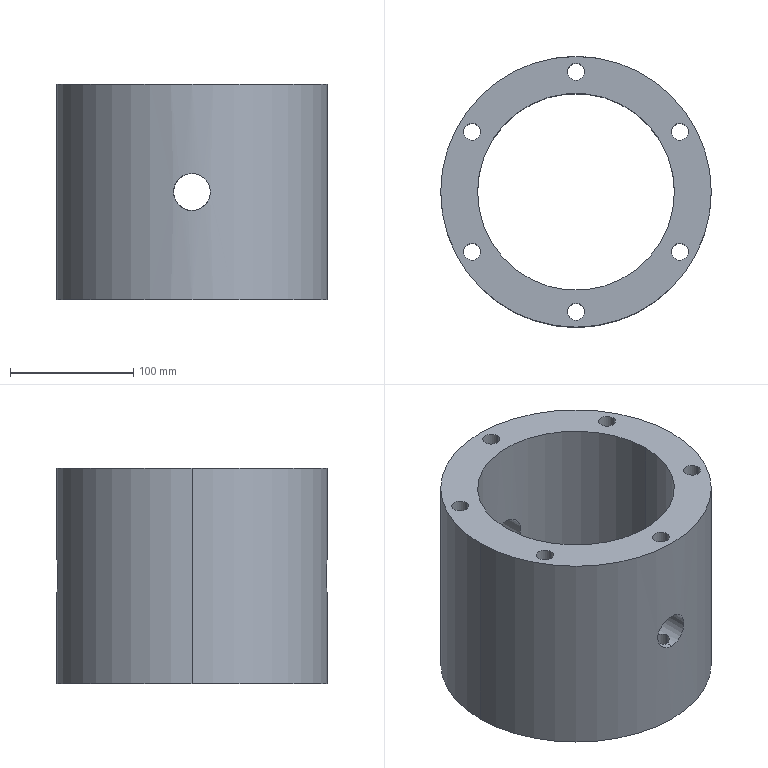Part | SolidWorks | features Extrusion 1, ICE 1 | 1 solid | 26 faces | box 220 x 220 x 175 mm | volume 2942854 mm3 | cylinder 24 | plane 2 | commonest cylinder face diameters 13.8 x16 30 x4 160 x2 220 x2